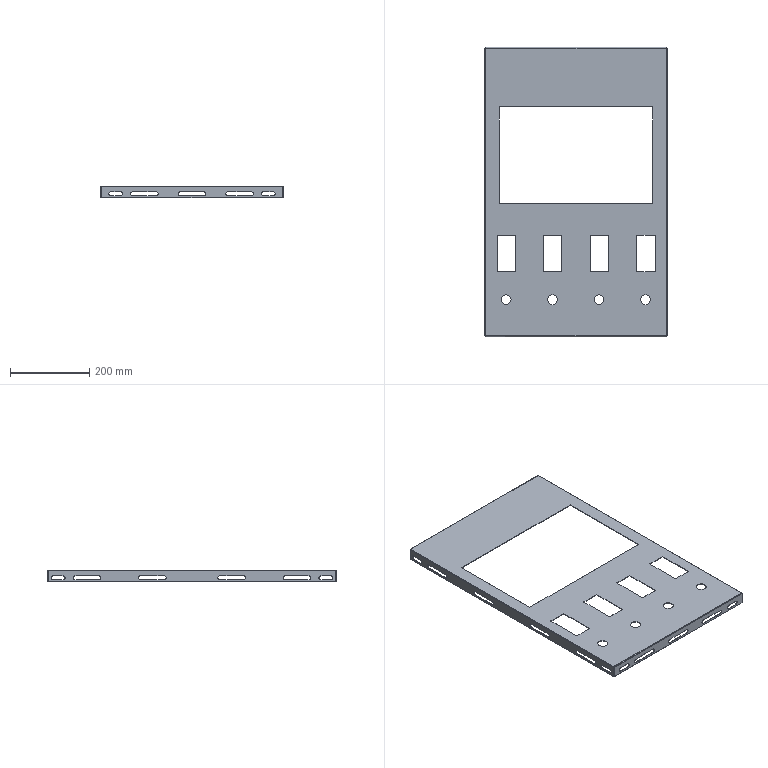Part | SolidWorks | features ICE 3, EdgeFlange 1, FlatPattern 1, SMBaseFlange 1, SheetMetal 1 | 1 solid | 154 faces | box 459 x 729 x 30 mm | volume 412274 mm3 | plane 86 | cylinder 60 | spline 8 | commonest cylinder face diameters 10 x44 25 x8 1 x4 4 x4